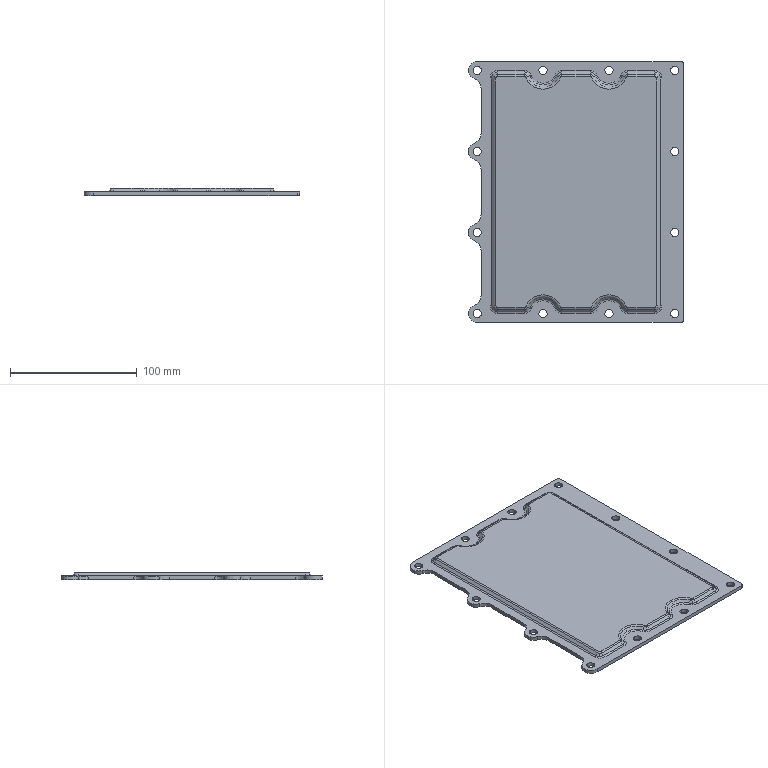Part | SolidWorks | features BaseBody 1 | 1 solid | 232 faces | box 170 x 206 x 6 mm | volume 103348 mm3 | cylinder 71 | cone 61 | torus 51 | plane 26 | sphere 18 | spline 5 | commonest cylinder face diameters 4 x37 6.5 x24 16 x6 14 x4